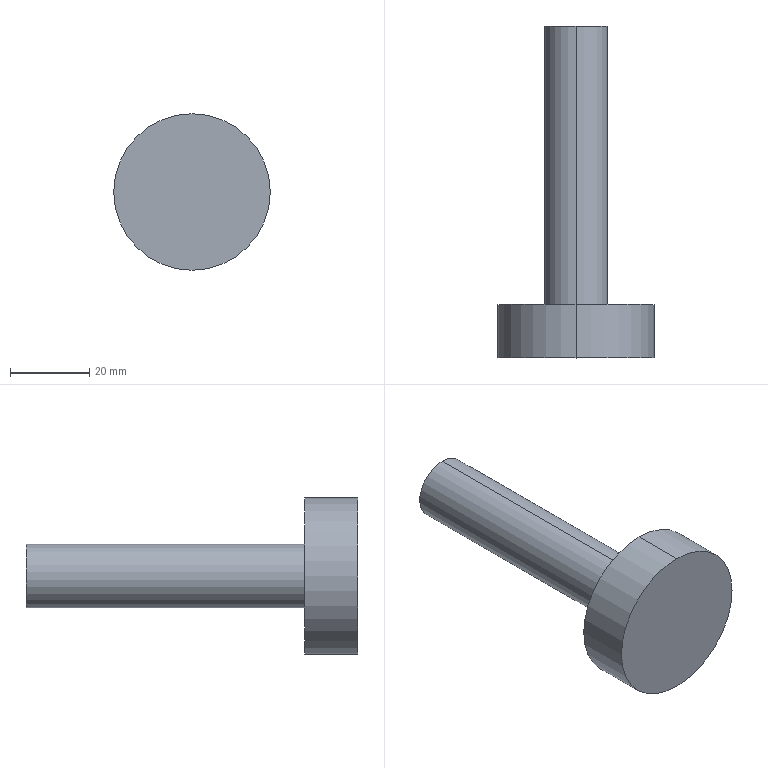Part | SolidWorks | features BaseBody 1 | 1 solid | 17 faces | box 39.6 x 84 x 39.6 mm | volume 30608 mm3 | cylinder 8 | plane 5 | cone 4 | commonest cylinder face diameters 13 x2 14 x2 16 x2 39.6 x2
STEP:
#1=CARTESIAN_POINT('',(0.,13.5,8.));
#2=VERTEX_POINT('',#1);
#3=CARTESIAN_POINT('',(0.,13.5,-8.));
#4=VERTEX_POINT('',#3);
#5=CARTESIAN_POINT('',(0.,13.5,0.));
#6=DIRECTION('',(0.,1.,0.));
#7=DIRECTION('',(0.,0.,1.));
#8=AXIS2_PLACEMENT_3D('',#5,#6,#7);
#9=CIRCLE('',#8,8.);
#10=EDGE_CURVE('',#2,#4,#9,.T.);
#11=ORIENTED_EDGE('',*,*,#10,.T.);
#12=CARTESIAN_POINT('',(0.,84.,-8.));
#13=VERTEX_POINT('',#12);
#14=CARTESIAN_POINT('',(0.,0.,-8.));
#15=DIRECTION('',(0.,1.,0.));
#16=VECTOR('',#15,1000.);
#17=LINE('',#14,#16);
#18=EDGE_CURVE('',#4,#13,#17,.T.);
#19=ORIENTED_EDGE('',*,*,#18,.T.);
#20=CARTESIAN_POINT('',(0.,84.,8.));
#21=VERTEX_POINT('',#20);
#22=CARTESIAN_POINT('',(0.,84.,0.));
#23=DIRECTION('',(0.,-1.,0.));
#24=DIRECTION('',(0.,0.,1.));
#25=AXIS2_PLACEMENT_3D('',#22,#23,#24);
#26=CIRCLE('',#25,8.);
#27=EDGE_CURVE('',#13,#21,#26,.T.);
#28=ORIENTED_EDGE('',*,*,#27,.T.);
#29=CARTESIAN_POINT('',(0.,0.,8.));
#30=DIRECTION('',(0.,1.,0.));
#31=VECTOR('',#30,1000.);
#32=LINE('',#29,#31);
#33=EDGE_CURVE('',#2,#21,#32,.T.);
#34=ORIENTED_EDGE('',*,*,#33,.F.);
#35=EDGE_LOOP('',(#11,#19,#28,#34));
#36=FACE_OUTER_BOUND('',#35,.T.);
#37=CARTESIAN_POINT('',(0.,0.,0.));
#38=DIRECTION('',(0.,1.,0.));
#39=DIRECTION('',(0.,0.,1.));
#40=AXIS2_PLACEMENT_3D('',#37,#38,#39);
#41=CYLINDRICAL_SURFACE('',#40,8.);
#42=ADVANCED_FACE('',(#36),#41,.T.);
#43=CARTESIAN_POINT('',(0.,83.5,-7.));
#44=VERTEX_POINT('',#43);
#45=CARTESIAN_POINT('',(0.,83.5,7.));
#46=VERTEX_POINT('',#45);
#47=CARTESIAN_POINT('',(0.,83.5,0.));
#48=DIRECTION('',(0.,1.,0.));
#49=DIRECTION('',(0.,0.,1.));
#50=AXIS2_PLACEMENT_3D('',#47,#48,#49);
#51=CIRCLE('',#50,7.);
#52=EDGE_CURVE('',#44,#46,#51,.T.);
#53=ORIENTED_EDGE('',*,*,#52,.F.);
#54=CARTESIAN_POINT('',(0.,84.,-7.5));
#55=VERTEX_POINT('',#54);
#56=CARTESIAN_POINT('',(0.,84.,-7.5));
#57=DIRECTION('',(0.,0.7071,-0.7071));
#58=VECTOR('',#57,1000.);
#59=LINE('',#56,#58);
#60=EDGE_CURVE('',#44,#55,#59,.T.);
#61=ORIENTED_EDGE('',*,*,#60,.T.);
#62=CARTESIAN_POINT('',(0.,84.,7.5));
#63=VERTEX_POINT('',#62);
#64=CARTESIAN_POINT('',(0.,84.,0.));
#65=DIRECTION('',(0.,1.,0.));
#66=DIRECTION('',(0.,0.,1.));
#67=AXIS2_PLACEMENT_3D('',#64,#65,#66);
#68=CIRCLE('',#67,7.5);
#69=EDGE_CURVE('',#55,#63,#68,.T.);
#70=ORIENTED_EDGE('',*,*,#69,.T.);
#71=CARTESIAN_POINT('',(0.,84.,7.5));
#72=DIRECTION('',(0.,0.7071,0.7071));
#73=VECTOR('',#72,1000.);
#74=LINE('',#71,#73);
#75=EDGE_CURVE('',#46,#63,#74,.T.);
#76=ORIENTED_EDGE('',*,*,#75,.F.);
#77=EDGE_LOOP('',(#53,#61,#70,#76));
#78=FACE_OUTER_BOUND('',#77,.T.);
#79=CARTESIAN_POINT('',(0.,84.,0.));
#80=DIRECTION('',(0.,1.,0.));
#81=DIRECTION('',(0.,0.,1.));
#82=AXIS2_PLACEMENT_3D('',#79,#80,#81);
#83=CONICAL_SURFACE('',#82,7.5,0.7854);
#84=ADVANCED_FACE('',(#78),#83,.F.);
#85=CARTESIAN_POINT('',(0.,0.,19.8));
#86=VERTEX_POINT('',#85);
#87=CARTESIAN_POINT('',(0.,0.,-19.8));
#88=VERTEX_POINT('',#87);
#89=CARTESIAN_POINT('',(0.,0.,0.));
#90=DIRECTION('',(0.,1.,0.));
#91=DIRECTION('',(0.,0.,1.));
#92=AXIS2_PLACEMENT_3D('',#89,#90,#91);
#93=CIRCLE('',#92,19.8);
#94=EDGE_CURVE('',#86,#88,#93,.T.);
#95=ORIENTED_EDGE('',*,*,#94,.T.);
#96=CARTESIAN_POINT('',(0.,13.5,-19.8));
#97=VERTEX_POINT('',#96);
#98=CARTESIAN_POINT('',(0.,0.,-19.8));
#99=DIRECTION('',(0.,1.,0.));
#100=VECTOR('',#99,1000.);
#101=LINE('',#98,#100);
#102=EDGE_CURVE('',#88,#97,#101,.T.);
#103=ORIENTED_EDGE('',*,*,#102,.T.);
#104=CARTESIAN_POINT('',(0.,13.5,19.8));
#105=VERTEX_POINT('',#104);
#106=CARTESIAN_POINT('',(0.,13.5,0.));
#107=DIRECTION('',(0.,-1.,0.));
#108=DIRECTION('',(0.,0.,1.));
#109=AXIS2_PLACEMENT_3D('',#106,#107,#108);
#110=CIRCLE('',#109,19.8);
#111=EDGE_CURVE('',#97,#105,#110,.T.);
#112=ORIENTED_EDGE('',*,*,#111,.T.);
#113=CARTESIAN_POINT('',(0.,0.,19.8));
#114=DIRECTION('',(0.,1.,0.));
#115=VECTOR('',#114,1000.);
#116=LINE('',#113,#115);
#117=EDGE_CURVE('',#86,#105,#116,.T.);
#118=ORIENTED_EDGE('',*,*,#117,.F.);
#119=EDGE_LOOP('',(#95,#103,#112,#118));
#120=FACE_OUTER_BOUND('',#119,.T.);
#121=CARTESIAN_POINT('',(0.,0.,0.));
#122=DIRECTION('',(0.,1.,0.));
#123=DIRECTION('',(0.,0.,1.));
#124=AXIS2_PLACEMENT_3D('',#121,#122,#123);
#125=CYLINDRICAL_SURFACE('',#124,19.8);
#126=ADVANCED_FACE('',(#120),#125,.T.);
#127=ORIENTED_EDGE('',*,*,#52,.T.);
#128=CARTESIAN_POINT('',(0.,78.5,7.));
#129=VERTEX_POINT('',#128);
#130=CARTESIAN_POINT('',(0.,84.,7.));
#131=DIRECTION('',(0.,-1.,0.));
#132=VECTOR('',#131,1000.);
#133=LINE('',#130,#132);
#134=EDGE_CURVE('',#46,#129,#133,.T.);
#135=ORIENTED_EDGE('',*,*,#134,.T.);
#136=CARTESIAN_POINT('',(0.,78.5,-7.));
#137=VERTEX_POINT('',#136);
#138=CARTESIAN_POINT('',(0.,78.5,0.));
#139=DIRECTION('',(0.,1.,0.));
#140=DIRECTION('',(0.,0.,-1.));
#141=AXIS2_PLACEMENT_3D('',#138,#139,#140);
#142=CIRCLE('',#141,7.);
#143=EDGE_CURVE('',#137,#129,#142,.T.);
#144=ORIENTED_EDGE('',*,*,#143,.F.);
#145=CARTESIAN_POINT('',(0.,84.,-7.));
#146=DIRECTION('',(0.,-1.,0.));
#147=VECTOR('',#146,1000.);
#148=LINE('',#145,#147);
#149=EDGE_CURVE('',#44,#137,#148,.T.);
#150=ORIENTED_EDGE('',*,*,#149,.F.);
#151=EDGE_LOOP('',(#127,#135,#144,#150));
#152=FACE_OUTER_BOUND('',#151,.T.);
#153=CARTESIAN_POINT('',(0.,84.,0.));
#154=DIRECTION('',(0.,-1.,0.));
#155=DIRECTION('',(0.,0.,-1.));
#156=AXIS2_PLACEMENT_3D('',#153,#154,#155);
#157=CYLINDRICAL_SURFACE('',#156,7.);
#158=ADVANCED_FACE('',(#152),#157,.F.);
#159=CARTESIAN_POINT('',(0.,83.,-6.5));
#160=VERTEX_POINT('',#159);
#161=CARTESIAN_POINT('',(0.,83.,6.5));
#162=VERTEX_POINT('',#161);
#163=CARTESIAN_POINT('',(0.,83.,0.));
#164=DIRECTION('',(0.,-1.,0.));
#165=DIRECTION('',(0.,0.,-1.));
#166=AXIS2_PLACEMENT_3D('',#163,#164,#165);
#167=CIRCLE('',#166,6.5);
#168=EDGE_CURVE('',#160,#162,#167,.T.);
#169=ORIENTED_EDGE('',*,*,#168,.T.);
#170=CARTESIAN_POINT('',(0.,78.5,6.5));
#171=VERTEX_POINT('',#170);
#172=CARTESIAN_POINT('',(0.,84.,6.5));
#173=DIRECTION('',(0.,-1.,0.));
#174=VECTOR('',#173,1000.);
#175=LINE('',#172,#174);
#176=EDGE_CURVE('',#162,#171,#175,.T.);
#177=ORIENTED_EDGE('',*,*,#176,.T.);
#178=CARTESIAN_POINT('',(0.,78.5,-6.5));
#179=VERTEX_POINT('',#178);
#180=CARTESIAN_POINT('',(0.,78.5,0.));
#181=DIRECTION('',(0.,-1.,0.));
#182=DIRECTION('',(0.,0.,-1.));
#183=AXIS2_PLACEMENT_3D('',#180,#181,#182);
#184=CIRCLE('',#183,6.5);
#185=EDGE_CURVE('',#179,#171,#184,.T.);
#186=ORIENTED_EDGE('',*,*,#185,.F.);
#187=CARTESIAN_POINT('',(0.,84.,-6.5));
#188=DIRECTION('',(0.,-1.,0.));
#189=VECTOR('',#188,1000.);
#190=LINE('',#187,#189);
#191=EDGE_CURVE('',#160,#179,#190,.T.);
#192=ORIENTED_EDGE('',*,*,#191,.F.);
#193=EDGE_LOOP('',(#169,#177,#186,#192));
#194=FACE_OUTER_BOUND('',#193,.T.);
#195=CARTESIAN_POINT('',(0.,84.,0.));
#196=DIRECTION('',(0.,-1.,0.));
#197=DIRECTION('',(0.,0.,-1.));
#198=AXIS2_PLACEMENT_3D('',#195,#196,#197);
#199=CYLINDRICAL_SURFACE('',#198,6.5);
#200=ADVANCED_FACE('',(#194),#199,.T.);
#201=CARTESIAN_POINT('',(0.,83.5,-6.));
#202=VERTEX_POINT('',#201);
#203=CARTESIAN_POINT('',(0.,83.5,6.));
#204=VERTEX_POINT('',#203);
#205=CARTESIAN_POINT('',(0.,83.5,0.));
#206=DIRECTION('',(0.,-1.,0.));
#207=DIRECTION('',(0.,0.,-1.));
#208=AXIS2_PLACEMENT_3D('',#205,#206,#207);
#209=CIRCLE('',#208,6.);
#210=EDGE_CURVE('',#202,#204,#209,.T.);
#211=ORIENTED_EDGE('',*,*,#210,.T.);
#212=CARTESIAN_POINT('',(0.,83.,6.5));
#213=DIRECTION('',(0.,-0.7071,0.7071));
#214=VECTOR('',#213,1000.);
#215=LINE('',#212,#214);
#216=EDGE_CURVE('',#204,#162,#215,.T.);
#217=ORIENTED_EDGE('',*,*,#216,.T.);
#218=ORIENTED_EDGE('',*,*,#168,.F.);
#219=CARTESIAN_POINT('',(0.,83.,-6.5));
#220=DIRECTION('',(0.,-0.7071,-0.7071));
#221=VECTOR('',#220,1000.);
#222=LINE('',#219,#221);
#223=EDGE_CURVE('',#202,#160,#222,.T.);
#224=ORIENTED_EDGE('',*,*,#223,.F.);
#225=EDGE_LOOP('',(#211,#217,#218,#224));
#226=FACE_OUTER_BOUND('',#225,.T.);
#227=CARTESIAN_POINT('',(0.,83.,0.));
#228=DIRECTION('',(0.,-1.,0.));
#229=DIRECTION('',(0.,0.,-1.));
#230=AXIS2_PLACEMENT_3D('',#227,#228,#229);
#231=CONICAL_SURFACE('',#230,6.5,0.7854);
#232=ADVANCED_FACE('',(#226),#231,.T.);
#233=ORIENTED_EDGE('',*,*,#18,.F.);
#234=CARTESIAN_POINT('',(0.,13.5,0.));
#235=DIRECTION('',(0.,1.,0.));
#236=DIRECTION('',(0.,0.,1.));
#237=AXIS2_PLACEMENT_3D('',#234,#235,#236);
#238=CIRCLE('',#237,8.);
#239=EDGE_CURVE('',#4,#2,#238,.T.);
#240=ORIENTED_EDGE('',*,*,#239,.T.);
#241=ORIENTED_EDGE('',*,*,#33,.T.);
#242=CARTESIAN_POINT('',(0.,84.,0.));
#243=DIRECTION('',(0.,-1.,0.));
#244=DIRECTION('',(0.,0.,1.));
#245=AXIS2_PLACEMENT_3D('',#242,#243,#244);
#246=CIRCLE('',#245,8.);
#247=EDGE_CURVE('',#21,#13,#246,.T.);
#248=ORIENTED_EDGE('',*,*,#247,.T.);
#249=EDGE_LOOP('',(#233,#240,#241,#248));
#250=FACE_OUTER_BOUND('',#249,.T.);
#251=CARTESIAN_POINT('',(0.,0.,0.));
#252=DIRECTION('',(0.,1.,0.));
#253=DIRECTION('',(0.,0.,1.));
#254=AXIS2_PLACEMENT_3D('',#251,#252,#253);
#255=CYLINDRICAL_SURFACE('',#254,8.);
#256=ADVANCED_FACE('',(#250),#255,.T.);
#257=ORIENTED_EDGE('',*,*,#247,.F.);
#258=ORIENTED_EDGE('',*,*,#27,.F.);
#259=EDGE_LOOP('',(#257,#258));
#260=FACE_OUTER_BOUND('',#259,.T.);
#261=CARTESIAN_POINT('',(0.,84.,0.));
#262=DIRECTION('',(0.,1.,0.));
#263=DIRECTION('',(0.,0.,1.));
#264=AXIS2_PLACEMENT_3D('',#261,#262,#263);
#265=CIRCLE('',#264,7.5);
#266=EDGE_CURVE('',#63,#55,#265,.T.);
#267=ORIENTED_EDGE('',*,*,#266,.F.);
#268=ORIENTED_EDGE('',*,*,#69,.F.);
#269=EDGE_LOOP('',(#267,#268));
#270=FACE_BOUND('',#269,.T.);
#271=CARTESIAN_POINT('',(11.,84.,9.5));
#272=DIRECTION('',(0.,-1.,0.));
#273=DIRECTION('',(0.,0.,-1.));
#274=AXIS2_PLACEMENT_3D('',#271,#272,#273);
#275=PLANE('',#274);
#276=ADVANCED_FACE('',(#260,#270),#275,.F.);
#277=CARTESIAN_POINT('',(0.,13.5,0.));
#278=DIRECTION('',(0.,-1.,0.));
#279=DIRECTION('',(0.,0.,1.));
#280=AXIS2_PLACEMENT_3D('',#277,#278,#279);
#281=CIRCLE('',#280,19.8);
#282=EDGE_CURVE('',#105,#97,#281,.T.);
#283=ORIENTED_EDGE('',*,*,#282,.F.);
#284=ORIENTED_EDGE('',*,*,#111,.F.);
#285=EDGE_LOOP('',(#283,#284));
#286=FACE_OUTER_BOUND('',#285,.T.);
#287=ORIENTED_EDGE('',*,*,#10,.F.);
#288=ORIENTED_EDGE('',*,*,#239,.F.);
#289=EDGE_LOOP('',(#287,#288));
#290=FACE_BOUND('',#289,.T.);
#291=CARTESIAN_POINT('',(8.,13.5,0.));
#292=DIRECTION('',(0.,-1.,0.));
#293=DIRECTION('',(0.,0.,-1.));
#294=AXIS2_PLACEMENT_3D('',#291,#292,#293);
#295=PLANE('',#294);
#296=ADVANCED_FACE('',(#286,#290),#295,.F.);
#297=ORIENTED_EDGE('',*,*,#60,.F.);
#298=CARTESIAN_POINT('',(0.,83.5,0.));
#299=DIRECTION('',(0.,1.,0.));
#300=DIRECTION('',(0.,0.,1.));
#301=AXIS2_PLACEMENT_3D('',#298,#299,#300);
#302=CIRCLE('',#301,7.);
#303=EDGE_CURVE('',#46,#44,#302,.T.);
#304=ORIENTED_EDGE('',*,*,#303,.F.);
#305=ORIENTED_EDGE('',*,*,#75,.T.);
#306=ORIENTED_EDGE('',*,*,#266,.T.);
#307=EDGE_LOOP('',(#297,#304,#305,#306));
#308=FACE_OUTER_BOUND('',#307,.T.);
#309=CARTESIAN_POINT('',(0.,84.,0.));
#310=DIRECTION('',(0.,1.,0.));
#311=DIRECTION('',(0.,0.,1.));
#312=AXIS2_PLACEMENT_3D('',#309,#310,#311);
#313=CONICAL_SURFACE('',#312,7.5,0.7854);
#314=ADVANCED_FACE('',(#308),#313,.F.);
#315=ORIENTED_EDGE('',*,*,#102,.F.);
#316=CARTESIAN_POINT('',(0.,0.,0.));
#317=DIRECTION('',(0.,1.,0.));
#318=DIRECTION('',(0.,0.,1.));
#319=AXIS2_PLACEMENT_3D('',#316,#317,#318);
#320=CIRCLE('',#319,19.8);
#321=EDGE_CURVE('',#88,#86,#320,.T.);
#322=ORIENTED_EDGE('',*,*,#321,.T.);
#323=ORIENTED_EDGE('',*,*,#117,.T.);
#324=ORIENTED_EDGE('',*,*,#282,.T.);
#325=EDGE_LOOP('',(#315,#322,#323,#324));
#326=FACE_OUTER_BOUND('',#325,.T.);
#327=CARTESIAN_POINT('',(0.,0.,0.));
#328=DIRECTION('',(0.,1.,0.));
#329=DIRECTION('',(0.,0.,1.));
#330=AXIS2_PLACEMENT_3D('',#327,#328,#329);
#331=CYLINDRICAL_SURFACE('',#330,19.8);
#332=ADVANCED_FACE('',(#326),#331,.T.);
#333=ORIENTED_EDGE('',*,*,#134,.F.);
#334=ORIENTED_EDGE('',*,*,#303,.T.);
#335=ORIENTED_EDGE('',*,*,#149,.T.);
#336=CARTESIAN_POINT('',(0.,78.5,0.));
#337=DIRECTION('',(0.,1.,0.));
#338=DIRECTION('',(0.,0.,-1.));
#339=AXIS2_PLACEMENT_3D('',#336,#337,#338);
#340=CIRCLE('',#339,7.);
#341=EDGE_CURVE('',#129,#137,#340,.T.);
#342=ORIENTED_EDGE('',*,*,#341,.F.);
#343=EDGE_LOOP('',(#333,#334,#335,#342));
#344=FACE_OUTER_BOUND('',#343,.T.);
#345=CARTESIAN_POINT('',(0.,84.,0.));
#346=DIRECTION('',(0.,-1.,0.));
#347=DIRECTION('',(0.,0.,-1.));
#348=AXIS2_PLACEMENT_3D('',#345,#346,#347);
#349=CYLINDRICAL_SURFACE('',#348,7.);
#350=ADVANCED_FACE('',(#344),#349,.F.);
#351=ORIENTED_EDGE('',*,*,#94,.F.);
#352=ORIENTED_EDGE('',*,*,#321,.F.);
#353=EDGE_LOOP('',(#351,#352));
#354=FACE_OUTER_BOUND('',#353,.T.);
#355=CARTESIAN_POINT('',(19.8,0.,0.));
#356=DIRECTION('',(0.,1.,0.));
#357=DIRECTION('',(0.,0.,1.));
#358=AXIS2_PLACEMENT_3D('',#355,#356,#357);
#359=PLANE('',#358);
#360=ADVANCED_FACE('',(#354),#359,.F.);
#361=ORIENTED_EDGE('',*,*,#143,.T.);
#362=ORIENTED_EDGE('',*,*,#341,.T.);
#363=EDGE_LOOP('',(#361,#362));
#364=FACE_OUTER_BOUND('',#363,.T.);
#365=ORIENTED_EDGE('',*,*,#185,.T.);
#366=CARTESIAN_POINT('',(0.,78.5,0.));
#367=DIRECTION('',(0.,-1.,0.));
#368=DIRECTION('',(0.,0.,-1.));
#369=AXIS2_PLACEMENT_3D('',#366,#367,#368);
#370=CIRCLE('',#369,6.5);
#371=EDGE_CURVE('',#171,#179,#370,.T.);
#372=ORIENTED_EDGE('',*,*,#371,.T.);
#373=EDGE_LOOP('',(#365,#372));
#374=FACE_BOUND('',#373,.T.);
#375=CARTESIAN_POINT('',(-6.5,78.5,0.));
#376=DIRECTION('',(0.,1.,0.));
#377=DIRECTION('',(0.,0.,1.));
#378=AXIS2_PLACEMENT_3D('',#375,#376,#377);
#379=PLANE('',#378);
#380=ADVANCED_FACE('',(#364,#374),#379,.T.);
#381=ORIENTED_EDGE('',*,*,#176,.F.);
#382=CARTESIAN_POINT('',(0.,83.,0.));
#383=DIRECTION('',(0.,-1.,0.));
#384=DIRECTION('',(0.,0.,-1.));
#385=AXIS2_PLACEMENT_3D('',#382,#383,#384);
#386=CIRCLE('',#385,6.5);
#387=EDGE_CURVE('',#162,#160,#386,.T.);
#388=ORIENTED_EDGE('',*,*,#387,.T.);
#389=ORIENTED_EDGE('',*,*,#191,.T.);
#390=ORIENTED_EDGE('',*,*,#371,.F.);
#391=EDGE_LOOP('',(#381,#388,#389,#390));
#392=FACE_OUTER_BOUND('',#391,.T.);
#393=CARTESIAN_POINT('',(0.,84.,0.));
#394=DIRECTION('',(0.,-1.,0.));
#395=DIRECTION('',(0.,0.,-1.));
#396=AXIS2_PLACEMENT_3D('',#393,#394,#395);
#397=CYLINDRICAL_SURFACE('',#396,6.5);
#398=ADVANCED_FACE('',(#392),#397,.T.);
#399=ORIENTED_EDGE('',*,*,#216,.F.);
#400=CARTESIAN_POINT('',(0.,83.5,0.));
#401=DIRECTION('',(0.,-1.,0.));
#402=DIRECTION('',(0.,0.,-1.));
#403=AXIS2_PLACEMENT_3D('',#400,#401,#402);
#404=CIRCLE('',#403,6.);
#405=EDGE_CURVE('',#204,#202,#404,.T.);
#406=ORIENTED_EDGE('',*,*,#405,.T.);
#407=ORIENTED_EDGE('',*,*,#223,.T.);
#408=ORIENTED_EDGE('',*,*,#387,.F.);
#409=EDGE_LOOP('',(#399,#406,#407,#408));
#410=FACE_OUTER_BOUND('',#409,.T.);
#411=CARTESIAN_POINT('',(0.,83.,0.));
#412=DIRECTION('',(0.,-1.,0.));
#413=DIRECTION('',(0.,0.,-1.));
#414=AXIS2_PLACEMENT_3D('',#411,#412,#413);
#415=CONICAL_SURFACE('',#414,6.5,0.7854);
#416=ADVANCED_FACE('',(#410),#415,.T.);
#417=ORIENTED_EDGE('',*,*,#210,.F.);
#418=ORIENTED_EDGE('',*,*,#405,.F.);
#419=EDGE_LOOP('',(#417,#418));
#420=FACE_OUTER_BOUND('',#419,.T.);
#421=CARTESIAN_POINT('',(0.,83.5,0.));
#422=DIRECTION('',(0.,1.,0.));
#423=DIRECTION('',(0.,0.,1.));
#424=AXIS2_PLACEMENT_3D('',#421,#422,#423);
#425=PLANE('',#424);
#426=ADVANCED_FACE('',(#420),#425,.T.);
#427=CLOSED_SHELL('',(#42,#84,#126,#158,#200,#232,#256,#276,#296,#314,#332,#350,#360,#380,#398,#416,#426));
#428=MANIFOLD_SOLID_BREP('',#427);
#429=CARTESIAN_POINT('',(0.,0.,0.));
#430=DIRECTION('',(0.,0.,1.));
#431=DIRECTION('',(1.,0.,0.));
#432=AXIS2_PLACEMENT_3D('',#429,#430,#431);
#433=(LENGTH_UNIT()NAMED_UNIT(*)SI_UNIT(.MILLI.,.METRE.));
#434=UNCERTAINTY_MEASURE_WITH_UNIT(LENGTH_MEASURE(0.00001),#433,'','');
#435=(NAMED_UNIT(*)PLANE_ANGLE_UNIT()SI_UNIT($,.RADIAN.));
#436=(NAMED_UNIT(*)SI_UNIT($,.STERADIAN.)SOLID_ANGLE_UNIT());
#437=(GEOMETRIC_REPRESENTATION_CONTEXT(3)GLOBAL_UNCERTAINTY_ASSIGNED_CONTEXT((#434))GLOBAL_UNIT_ASSIGNED_CONTEXT((#433,#435,#436))REPRESENTATION_CONTEXT('',''));
#438=ADVANCED_BREP_SHAPE_REPRESENTATION('',(#428,#432),#437);